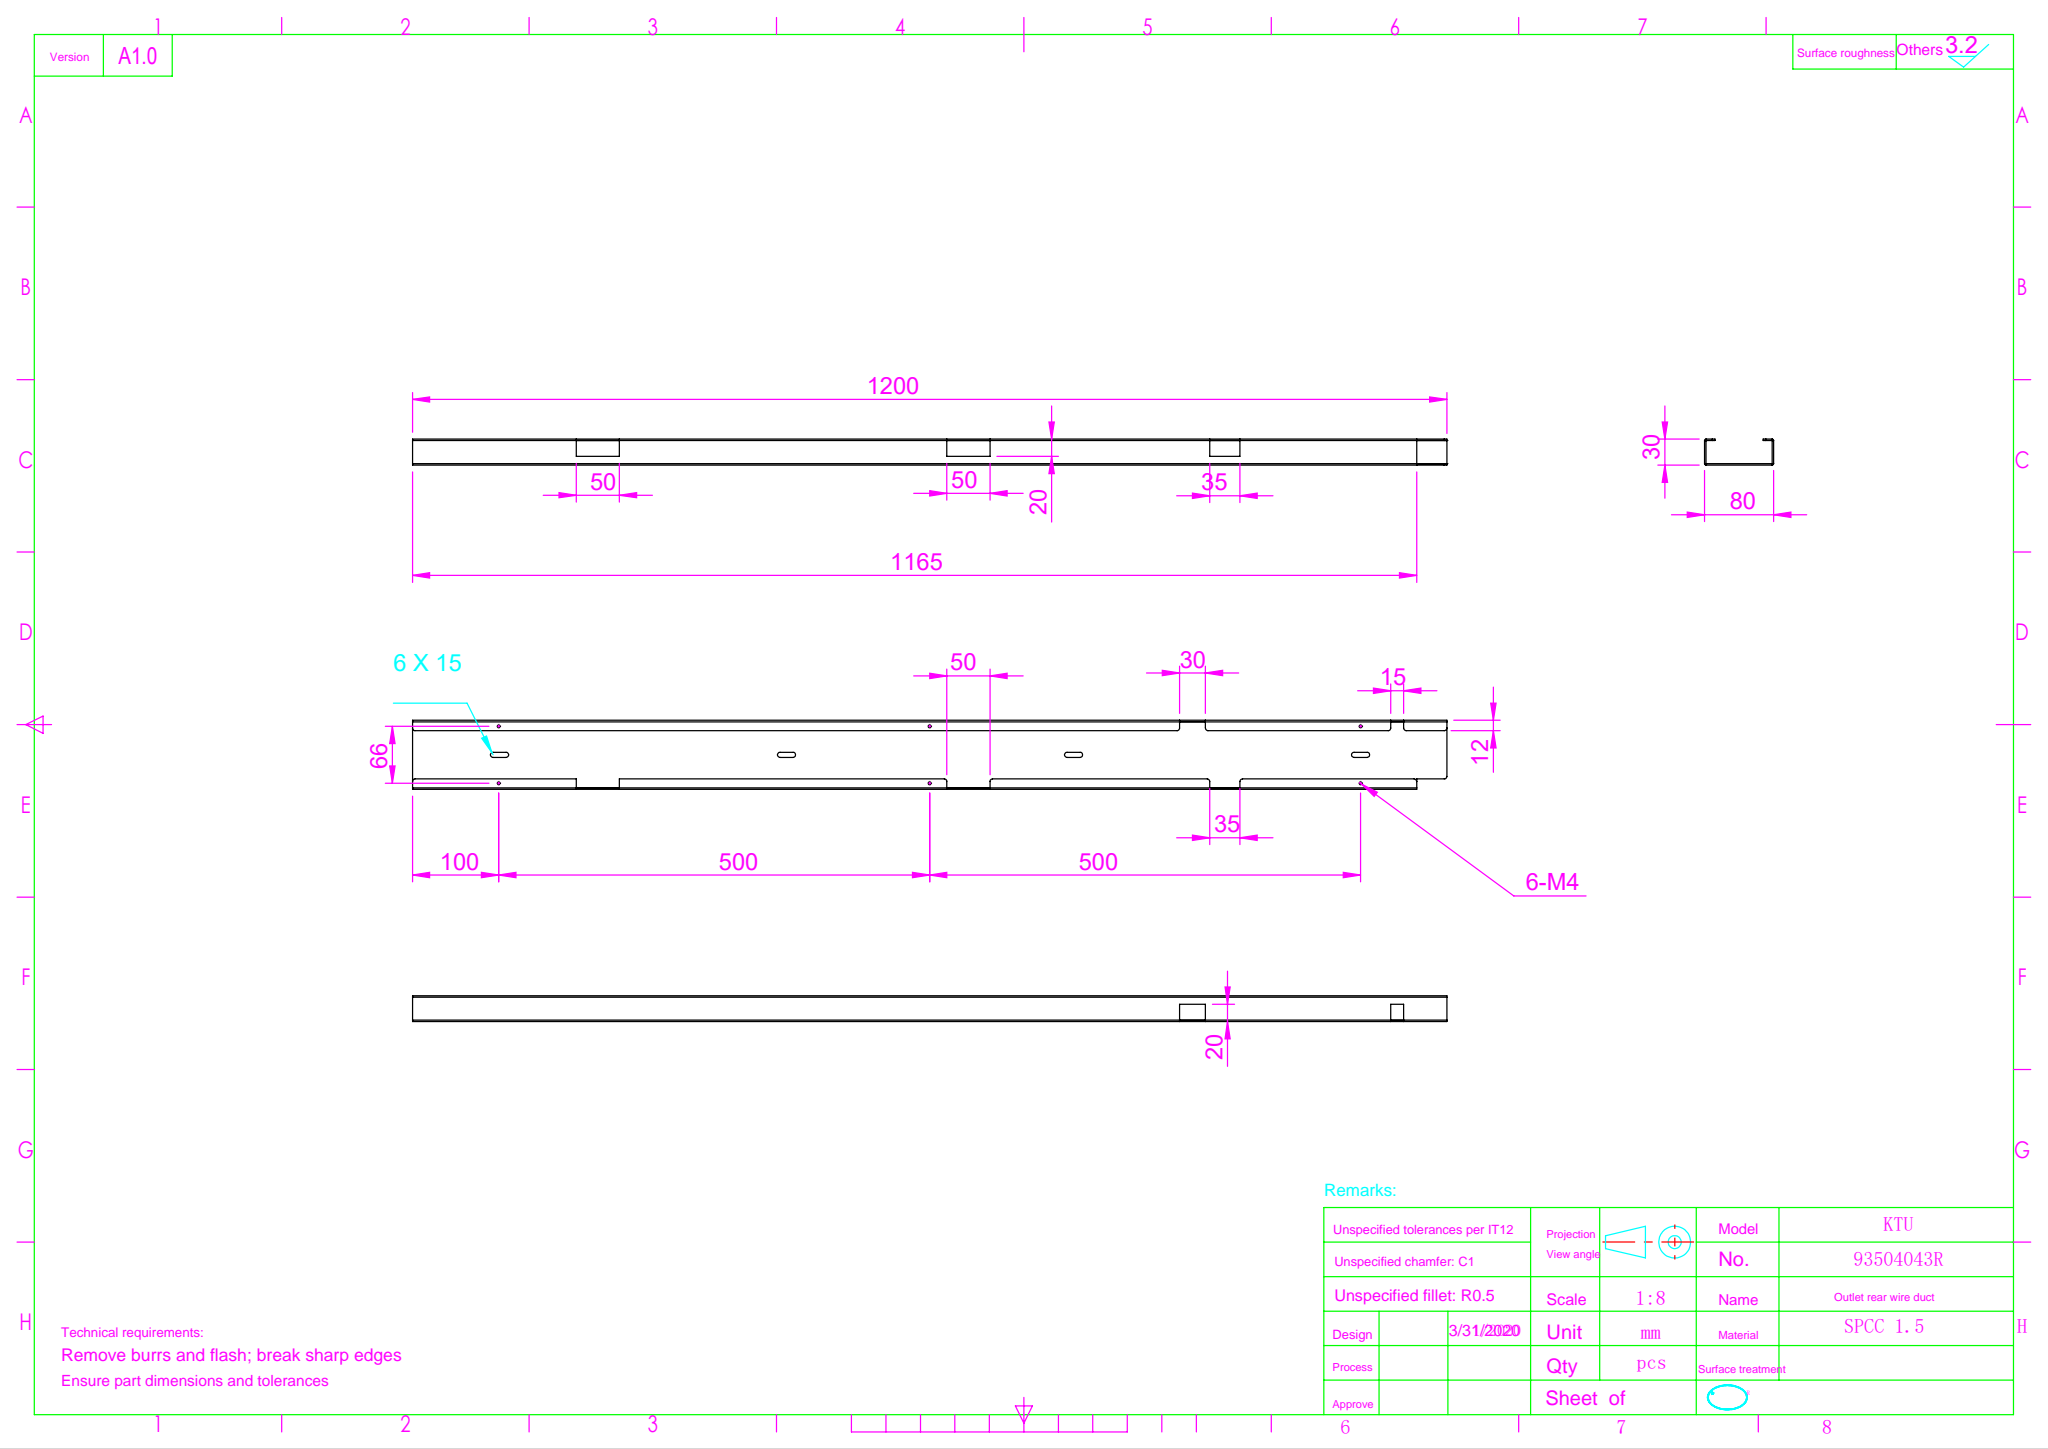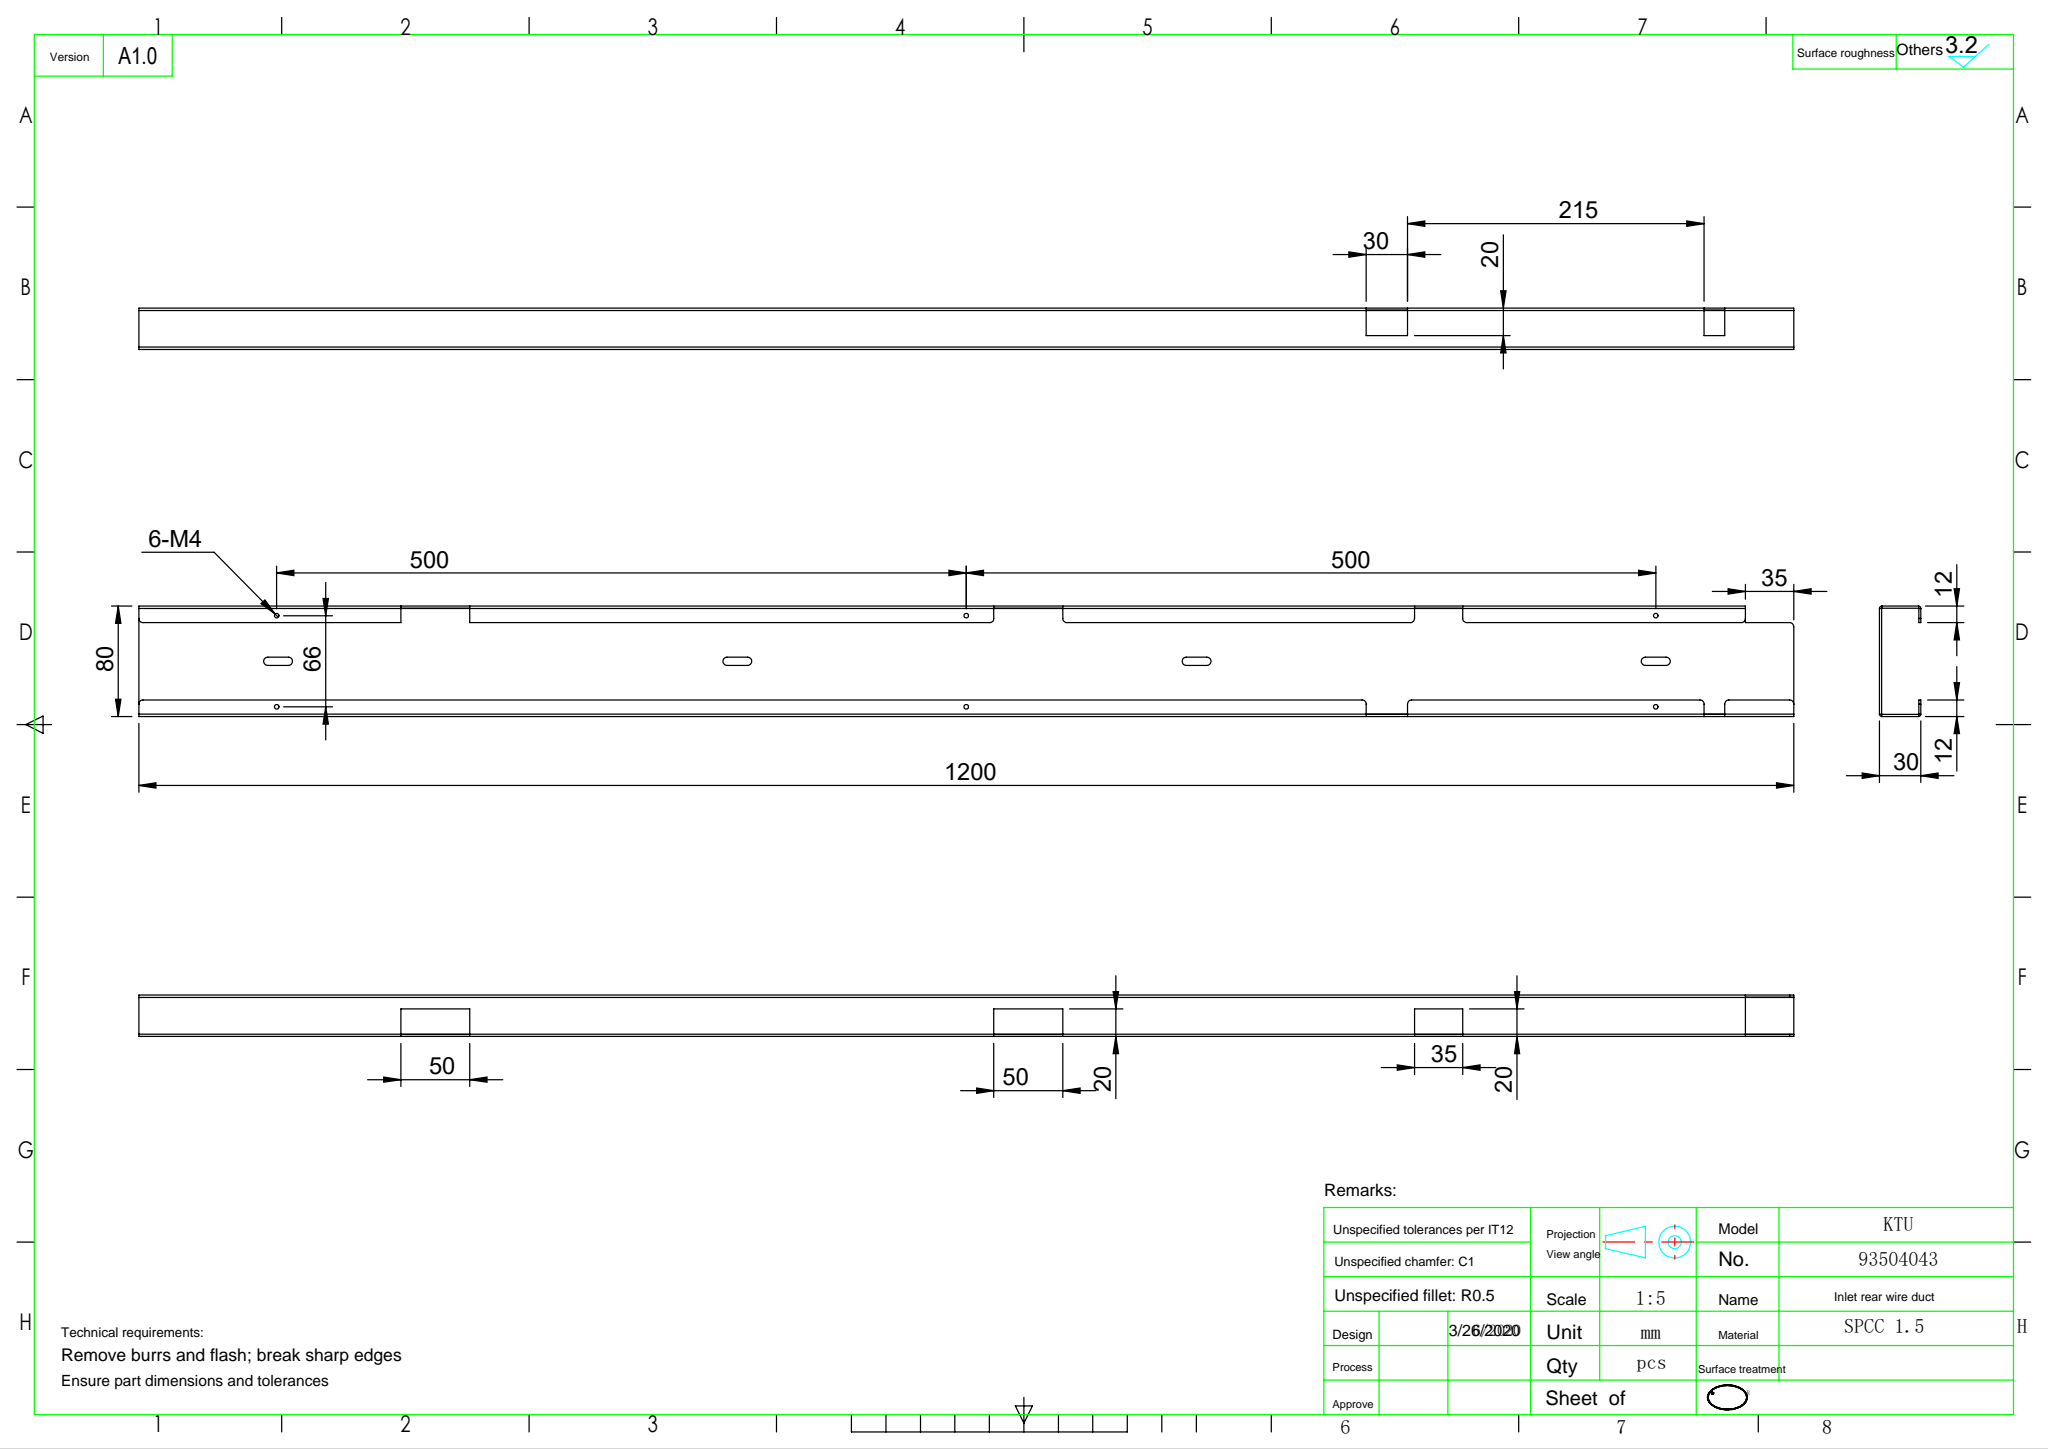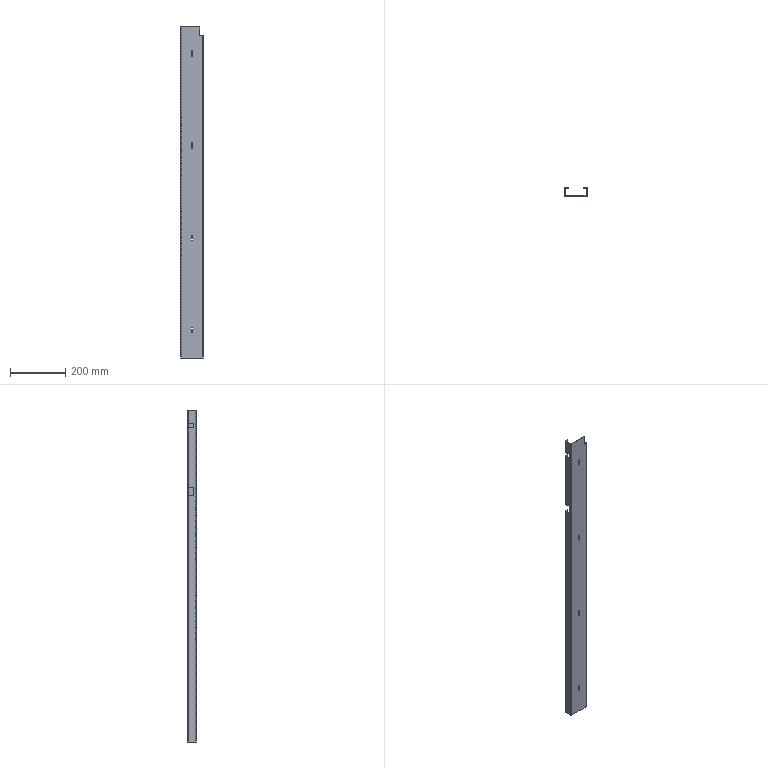Part | SolidWorks | features ICE 5, LPattern 2, Fillet 1, FlatPattern 1, HoleWzd 1, SMBaseFlange 1, SheetMetal 1 | 1 solid | 121 faces | box 80 x 30 x 1200 mm | volume 269880 mm3 | plane 66 | cylinder 55 | commonest cylinder face diameters 6 x25 3.3 x12 0.4 x9 3.4 x9